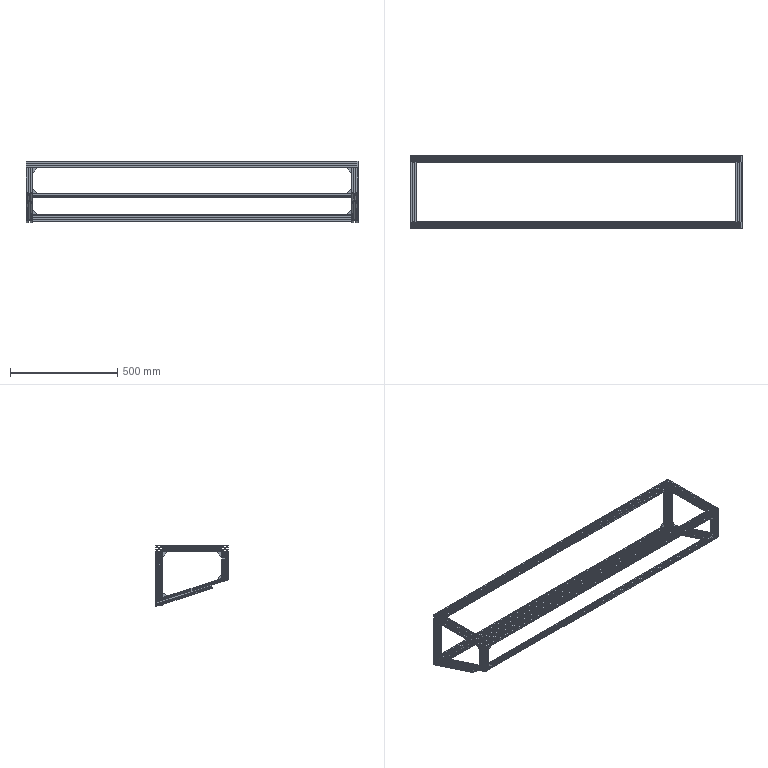Part | SolidWorks | features Gusset 16, WeldCornerFeat 2, 3DProfileFeature 1, ICE 1, WeldMemberFeat 1, WeldmentFeature 1 | 29 solids | 975 faces | box 1548 x 337.768 x 285.646 mm | volume 2440117 mm3 | plane 813 | cylinder 162 | commonest cylinder face diameters 3 x138 6.8 x24